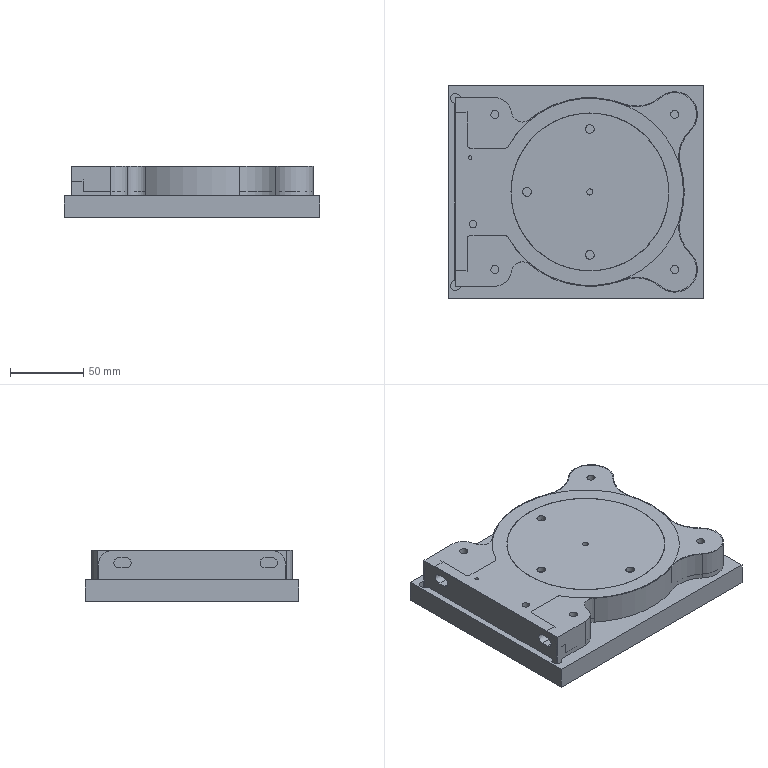CAM job | NX | 3-axis milling, drilling | part box 175 x 146 x 35 mm
Tools:
number,name,description,diameter,corner_radius,flute_length,length,flutes
2,D10,Milling Tool-5 Parameters,10.0,0.0,50.0,75.0,2
4,D6,Milling Tool-5 Parameters,6.0,0.0,30.0,50.0,2
5,D4,Milling Tool-5 Parameters,4.0,0.0,50.0,75.0,2
6,D3,Milling Tool-5 Parameters,3.0,0.0,50.0,75.0,2
7,D2,Milling Tool-5 Parameters,2.0,0.0,6.0,50.0,2
8,D1.5,Milling Tool-5 Parameters,1.5,0.0,6.0,75.0,2
12,DJ6,Milling Tool-5 Parameters,6.0,0.0,2.0,3.0,1
12,DJ8,Milling Tool-5 Parameters,8.0,0.0,3.0,4.0,2
16,Z4.3,Drilling Tool,4.2,0.0,35.0,50.0,2
24,R2,Milling Tool-5 Parameters,4.0,2.0,50.0,75.0,2
20,M5,Tap,5.0,0.0,20.0,100.0,2
Operations:
program,operation,operation_type,tool,method,geometry_group,spindle_rpm,surface_speed,feed_per_tooth,feed_cut,feed_plunge,cut_length_mm,path_length_mm,cut_time_min,machine_time_min
1-1001,正面_COPY,FaceMilling,D10,METHOD,WORKPIECE一夹,8000.0,251.0,0.125,2000.0,100.0,3767.524,3807.224,1.884,1.888
1-1001,跟随部件_COPY_2,CavityMilling,D10,METHOD,WORKPIECE一夹,8000.0,251.0,0.25,4000.0,100.0,18225.406,35249.724,4.556,5.691
1-1001,跟随部件_COPY_2_COPY,CavityMilling,D10,METHOD,WORKPIECE一夹,8000.0,251.0,0.25,4000.0,100.0,22821.363,30228.345,5.705,6.199
1-1002,打点_COPY_COPY,Operation,DJ6,METHOD,WORKPIECE一夹,3000.0,56.0,0.0667,200.0,0.0,21.0,524.741,0.105,0.1554
1-1003,DRILLING_COPY_1,Operation,Z4.3,METHOD,WORKPIECE一夹,3000.0,56.0,0.0667,200.0,0.0,90.0,606.633,0.45,0.5017
1-1004,打点_COPY_COPY_COPY,Operation,DJ6,METHOD,WORKPIECE一夹,3000.0,56.0,0.0667,200.0,0.0,27.5,537.741,0.1375,0.1885
1-1004,倒角_COPY_1_COPY_2,PlanarMilling,DJ6,METHOD,WORKPIECE一夹,7500.0,94.0,0.2,1500.0,100.0,432.988,473.988,0.2887,0.2928
1-1004,倒角_COPY_1_COPY_2_COPY,PlanarMilling,DJ6,METHOD,WORKPIECE一夹,7500.0,94.0,0.2,1500.0,100.0,627.436,668.436,0.4183,0.4224
1-1005,DRILLING_COPY_1_COPY,Operation,M5,METHOD,WORKPIECE一夹,300.0,4.0,0.4,240.0,0.0,80.0,586.633,0.3333,0.384
1-1006,正面_COPY_COPY,FaceMilling,D10,METHOD,WORKPIECE一夹,8000.0,251.0,0.0938,1500.0,100.0,3767.524,3807.324,2.512,2.516
1-1006,跟随部件_COPY_1_COPY_1,CavityMilling,D10,METHOD,WORKPIECE一夹,8000.0,251.0,0.0938,1500.0,100.0,1353.549,1446.549,0.9024,0.9086
201,反面_COPY,FaceMilling,D10,METHOD,WORKPIECE二夹,8000.0,251.0,0.25,4000.0,100.0,12241.909,12787.517,3.061,3.115
201,反面_COPY_COPY,FaceMilling,D10,METHOD,WORKPIECE二夹,8000.0,251.0,0.125,2000.0,100.0,3851.143,3890.943,1.926,1.93
202,打点_COPY_COPY_COPY_1,Operation,DJ8,METHOD,WORKPIECE二夹,3000.0,56.0,0.0667,200.0,0.0,25.2,485.104,0.126,0.172
203,DRILLING_COPY_1_COPY_1,Operation,Z4.3,METHOD,WORKPIECE二夹,3000.0,56.0,0.0667,200.0,0.0,18.0,76.0,0.09,0.0958
203,DRILLING_COPY_1_COPY_1_COPY_1,Operation,Z4.3,METHOD,WORKPIECE二夹,3000.0,56.0,0.0667,200.0,0.0,72.0,567.486,0.36,0.4095
204,打点_COPY_COPY_COPY_COPY,Operation,DJ8,METHOD,WORKPIECE二夹,3000.0,56.0,0.0667,200.0,0.0,16.5,263.668,0.0825,0.1072
204,打点_COPY_COPY_COPY_COPY_COPY,Operation,DJ8,METHOD,WORKPIECE二夹,3000.0,56.0,0.0667,200.0,0.0,16.5,219.611,0.0825,0.1028
204,倒角_COPY_1_COPY_2_COPY_1,PlanarMilling,DJ8,METHOD,WORKPIECE二夹,7500.0,94.0,0.2,1500.0,100.0,631.577,672.577,0.4211,0.4252
205,DRILLING_COPY_1_COPY_COPY,Operation,M5,METHOD,WORKPIECE二夹,300.0,4.0,0.4,240.0,0.0,82.5,591.633,0.3438,0.3947
301,跟随部件_COPY_3,CavityMilling,D10,METHOD,WORKPIECE三夹,8000.0,251.0,0.25,4000.0,100.0,13334.964,13625.611,3.334,3.353
302,底壁_COPY_COPY_1,VolumeBased25DMillingOperation,D10,METHOD,WORKPIECE三夹,8500.0,267.0,0.0882,1500.0,100.0,3335.869,3384.869,2.224,2.229
302,外形分层_COPY_1_COPY_COPY,PlanarMilling,D10,METHOD,WORKPIECE三夹,8500.0,267.0,0.0882,1500.0,100.0,604.957,653.957,0.4033,0.4082
402,FACE_MILLING_COPY_COPY_1,FaceMilling,D10,METHOD,WORKPIECE四夹,8500.0,267.0,0.0882,1500.0,100.0,3469.965,3508.965,2.313,2.317
403,深度开粗_COPY,ZLevelMilling,D6,METHOD,WORKPIECE四夹,9000.0,169.0,0.1389,2500.0,100.0,3449.637,4603.968,1.38,1.495
403,跟随部件_COPY_4,CavityMilling,D6,METHOD,WORKPIECE四夹,8000.0,251.0,0.25,4000.0,100.0,3839.646,4251.869,0.9599,0.9874
403,底壁_COPY_COPY_COPY_2,VolumeBased25DMillingOperation,D6,METHOD,WORKPIECE四夹,10000.0,314.0,0.075,1500.0,100.0,43.425,123.025,0.0289,0.0369
403,深度光_COPY_1,ZLevelMilling,D6,METHOD,WORKPIECE四夹,8500.0,267.0,0.0882,1500.0,100.0,2968.358,3356.824,1.979,2.018
405,深度开粗_COPY_COPY_1,ZLevelMilling,D3,METHOD,WORKPIECE四夹,9000.0,169.0,0.1389,2500.0,100.0,2847.064,4651.513,1.139,1.319
405,底壁螺旋_COPY_COPY,VolumeBased25DMillingOperation,D3,METHOD,WORKPIECE四夹,9000.0,169.0,0.1389,2500.0,100.0,319.505,402.905,0.1278,0.1361
405,底壁_COPY_COPY_COPY_2_COPY,VolumeBased25DMillingOperation,D3,METHOD,WORKPIECE四夹,10000.0,314.0,0.075,1500.0,100.0,230.148,301.949,0.1534,0.1606
405,底壁_COPY_COPY_COPY_2_COPY_COPY,VolumeBased25DMillingOperation,D3,METHOD,WORKPIECE四夹,10000.0,314.0,0.075,1500.0,100.0,22.722,118.722,0.0151,0.0247
406,DRILLING_COPY_1_COPY_1_COPY,Operation,D2,METHOD,WORKPIECE四夹,3000.0,56.0,0.0667,200.0,0.0,26.5,93.0,0.1325,0.1392
51,FACE_MILLING_COPY_COPY_1_COPY,FaceMilling,D10,METHOD,WORKPIECE五夹_,8500.0,267.0,0.0882,1500.0,100.0,3469.965,3508.965,2.313,2.317
51,底壁_COPY_1,VolumeBased25DMillingOperation,D10,METHOD,WORKPIECE五夹_,8000.0,251.0,0.25,4000.0,100.0,402.749,694.949,0.1007,0.1299
51,跟随部件_COPY_1_COPY_2,CavityMilling,D10,METHOD,WORKPIECE五夹_,8500.0,267.0,0.0882,1500.0,100.0,1320.755,1457.255,0.8805,0.8896
51,跟随部件_COPY_1_COPY_2_COPY,CavityMilling,D10,METHOD,WORKPIECE五夹_,8500.0,267.0,0.0882,1500.0,100.0,1318.455,1490.955,0.879,0.8905
58,深度开粗_COPY_COPY_1_COPY,ZLevelMilling,D4,METHOD,WORKPIECE五夹_,9000.0,169.0,0.1389,2500.0,100.0,2030.579,3067.93,0.8122,0.916
52,孔铣_COPY_2,CylinderMilling,D3,METHOD,WORKPIECE五夹_,10000.0,125.0,0.075,1500.0,100.0,139.745,183.945,0.0932,0.0976
52,孔铣_COPY_2_COPY_1,CylinderMilling,D3,METHOD,WORKPIECE五夹_,10000.0,125.0,0.075,1500.0,100.0,477.354,727.977,0.3182,0.3433
56,孔铣_COPY_2_COPY,CylinderMilling,D1.5,METHOD,WORKPIECE五夹_,10000.0,125.0,0.075,1500.0,100.0,44.006,85.006,0.0293,0.0334
53,REGION_COPY_COPY_COPY,SurfaceContour,R2,METHOD,WORKPIECE五夹_,10000.0,314.0,0.25,5000.0,100.0,6222.468,6433.032,1.244,1.266
54,倒角_COPY_1_COPY_2_COPY_1_COPY_1,PlanarMilling,DJ6,METHOD,WORKPIECE五夹_,7500.0,94.0,0.2,1500.0,100.0,444.706,485.706,0.2965,0.3006
601,FACE_MILLING_COPY_COPY_2,FaceMilling,D10,METHOD,WORKPIECE6,8500.0,267.0,0.0882,1500.0,100.0,3469.965,3518.965,2.313,2.318
602,孔铣_COPY_1_COPY,CylinderMilling,D4,METHOD,WORKPIECE6,8000.0,100.0,0.0938,1500.0,100.0,380.047,691.858,0.2534,0.2845
603,倒角_COPY_COPY_1,PlanarMilling,DJ8,METHOD,WORKPIECE6,7500.0,94.0,0.2,1500.0,100.0,49.181,322.398,0.0328,0.0601
604,PLANAR_MILL_COPY_COPY_1,PlanarMilling,D4,METHOD,WORKPIECE6,8200.0,103.0,0.0366,600.0,100.0,78.786,383.869,0.1313,0.1618
701,FACE_MILLING_COPY_COPY_2_COPY,FaceMilling,D10,METHOD,WORKPIECE7,8000.0,251.0,0.0938,1500.0,100.0,3771.089,3810.089,2.514,2.518
701,底壁_COPY_2,VolumeBased25DMillingOperation,D10,METHOD,WORKPIECE7,8000.0,251.0,0.25,4000.0,100.0,3709.789,4400.036,0.9274,0.9965
702,孔铣_COPY_1_COPY_COPY,CylinderMilling,D4,METHOD,WORKPIECE7,8000.0,100.0,0.0938,1500.0,100.0,380.047,661.858,0.2534,0.2815
703,倒角_COPY_COPY_1_COPY,PlanarMilling,DJ8,METHOD,WORKPIECE7,7500.0,94.0,0.2,1500.0,100.0,49.181,292.398,0.0328,0.0571
703,倒角_COPY_COPY_1_COPY_COPY,PlanarMilling,DJ8,METHOD,WORKPIECE7,7500.0,94.0,0.2,1500.0,100.0,121.384,268.065,0.0809,0.0956
704,PLANAR_MILL_COPY_COPY_1_COPY,PlanarMilling,D4,METHOD,WORKPIECE7,8200.0,103.0,0.0366,600.0,100.0,78.786,353.869,0.1313,0.1588